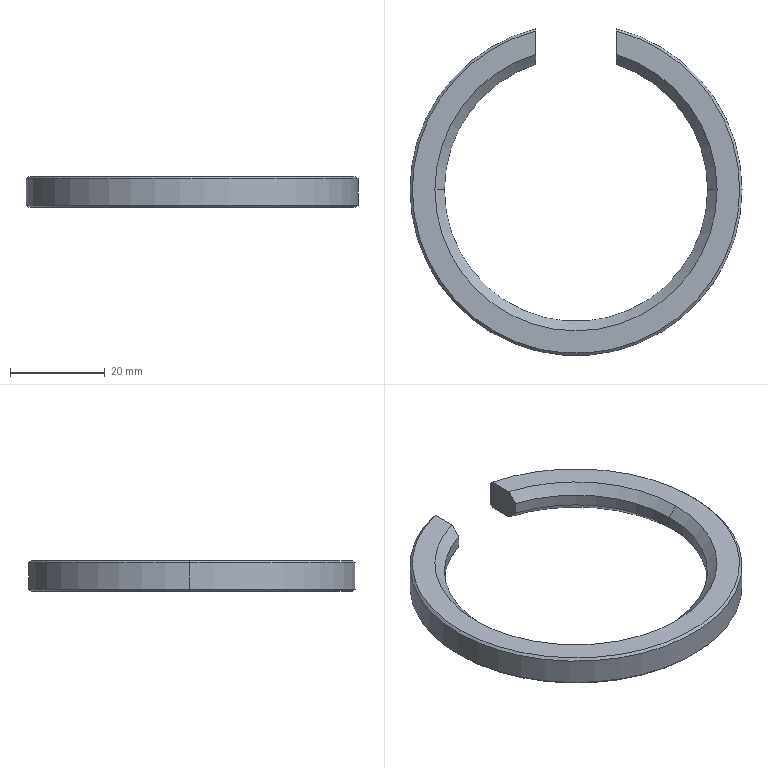Part | SolidWorks | features Chamfer 2, Extrusion 1, ICE 1 | 1 solid | 22 faces | box 70 x 68.952 x 6.5 mm | volume 7783 mm3 | cone 12 | cylinder 6 | plane 4 | commonest cylinder face diameters 55.5 x3 70 x3
STEP:
#1=CARTESIAN_POINT('',(34.5,0.,6.5));
#2=VERTEX_POINT('',#1);
#3=CARTESIAN_POINT('',(8.5,33.437,6.5));
#4=VERTEX_POINT('',#3);
#5=CARTESIAN_POINT('',(0.,0.,6.5));
#6=DIRECTION('',(0.,0.,1.));
#7=DIRECTION('',(1.,0.,0.));
#8=AXIS2_PLACEMENT_3D('',#5,#6,#7);
#9=CIRCLE('',#8,34.5);
#10=EDGE_CURVE('',#2,#4,#9,.T.);
#11=ORIENTED_EDGE('',*,*,#10,.F.);
#12=CARTESIAN_POINT('',(35.,0.,6.));
#13=VERTEX_POINT('',#12);
#14=CARTESIAN_POINT('',(34.5,0.,6.5));
#15=DIRECTION('',(0.7071,0.,-0.7071));
#16=VECTOR('',#15,1000.);
#17=LINE('',#14,#16);
#18=EDGE_CURVE('',#2,#13,#17,.T.);
#19=ORIENTED_EDGE('',*,*,#18,.T.);
#20=CARTESIAN_POINT('',(8.5,33.952,6.));
#21=VERTEX_POINT('',#20);
#22=CARTESIAN_POINT('',(0.,0.,6.));
#23=DIRECTION('',(0.,0.,-1.));
#24=DIRECTION('',(1.,0.,0.));
#25=AXIS2_PLACEMENT_3D('',#22,#23,#24);
#26=CIRCLE('',#25,35.);
#27=EDGE_CURVE('',#21,#13,#26,.T.);
#28=ORIENTED_EDGE('',*,*,#27,.F.);
#29=CARTESIAN_POINT('',(8.5,33.437,6.5));
#30=CARTESIAN_POINT('',(8.5,33.608,6.333));
#31=CARTESIAN_POINT('',(8.5,33.78,6.167));
#32=CARTESIAN_POINT('',(8.5,33.952,6.));
#33=B_SPLINE_CURVE_WITH_KNOTS('',3,(#29,#30,#31,#32),.UNSPECIFIED.,.F.,.F.,(4,4),(0.,0.0007183),.UNSPECIFIED.);
#34=EDGE_CURVE('',#4,#21,#33,.T.);
#35=ORIENTED_EDGE('',*,*,#34,.F.);
#36=EDGE_LOOP('',(#11,#19,#28,#35));
#37=FACE_OUTER_BOUND('',#36,.T.);
#38=CARTESIAN_POINT('',(0.,0.,6.5));
#39=DIRECTION('',(0.,0.,-1.));
#40=DIRECTION('',(-1.,0.,0.));
#41=AXIS2_PLACEMENT_3D('',#38,#39,#40);
#42=CONICAL_SURFACE('',#41,34.5,0.7854);
#43=ADVANCED_FACE('',(#37),#42,.T.);
#44=ORIENTED_EDGE('',*,*,#18,.F.);
#45=CARTESIAN_POINT('',(-34.5,0.,6.5));
#46=VERTEX_POINT('',#45);
#47=CARTESIAN_POINT('',(0.,0.,6.5));
#48=DIRECTION('',(0.,0.,1.));
#49=DIRECTION('',(1.,0.,0.));
#50=AXIS2_PLACEMENT_3D('',#47,#48,#49);
#51=CIRCLE('',#50,34.5);
#52=EDGE_CURVE('',#46,#2,#51,.T.);
#53=ORIENTED_EDGE('',*,*,#52,.F.);
#54=CARTESIAN_POINT('',(-35.,0.,6.));
#55=VERTEX_POINT('',#54);
#56=CARTESIAN_POINT('',(-34.5,0.,6.5));
#57=DIRECTION('',(-0.7071,0.,-0.7071));
#58=VECTOR('',#57,1000.);
#59=LINE('',#56,#58);
#60=EDGE_CURVE('',#46,#55,#59,.T.);
#61=ORIENTED_EDGE('',*,*,#60,.T.);
#62=CARTESIAN_POINT('',(0.,0.,6.));
#63=DIRECTION('',(0.,0.,-1.));
#64=DIRECTION('',(1.,0.,0.));
#65=AXIS2_PLACEMENT_3D('',#62,#63,#64);
#66=CIRCLE('',#65,35.);
#67=EDGE_CURVE('',#13,#55,#66,.T.);
#68=ORIENTED_EDGE('',*,*,#67,.F.);
#69=EDGE_LOOP('',(#44,#53,#61,#68));
#70=FACE_OUTER_BOUND('',#69,.T.);
#71=CARTESIAN_POINT('',(0.,0.,6.5));
#72=DIRECTION('',(0.,0.,-1.));
#73=DIRECTION('',(-1.,0.,0.));
#74=AXIS2_PLACEMENT_3D('',#71,#72,#73);
#75=CONICAL_SURFACE('',#74,34.5,0.7854);
#76=ADVANCED_FACE('',(#70),#75,.T.);
#77=CARTESIAN_POINT('',(-34.5,0.,0.));
#78=VERTEX_POINT('',#77);
#79=CARTESIAN_POINT('',(-8.5,33.437,0.));
#80=VERTEX_POINT('',#79);
#81=CARTESIAN_POINT('',(0.,0.,0.));
#82=DIRECTION('',(0.,0.,-1.));
#83=DIRECTION('',(1.,0.,0.));
#84=AXIS2_PLACEMENT_3D('',#81,#82,#83);
#85=CIRCLE('',#84,34.5);
#86=EDGE_CURVE('',#78,#80,#85,.T.);
#87=ORIENTED_EDGE('',*,*,#86,.F.);
#88=CARTESIAN_POINT('',(-35.,0.,0.5));
#89=VERTEX_POINT('',#88);
#90=CARTESIAN_POINT('',(-35.,0.,0.5));
#91=DIRECTION('',(-0.7071,0.,0.7071));
#92=VECTOR('',#91,1000.);
#93=LINE('',#90,#92);
#94=EDGE_CURVE('',#78,#89,#93,.T.);
#95=ORIENTED_EDGE('',*,*,#94,.T.);
#96=CARTESIAN_POINT('',(-8.5,33.952,0.5));
#97=VERTEX_POINT('',#96);
#98=CARTESIAN_POINT('',(0.,0.,0.5));
#99=DIRECTION('',(0.,0.,1.));
#100=DIRECTION('',(1.,0.,0.));
#101=AXIS2_PLACEMENT_3D('',#98,#99,#100);
#102=CIRCLE('',#101,35.);
#103=EDGE_CURVE('',#97,#89,#102,.T.);
#104=ORIENTED_EDGE('',*,*,#103,.F.);
#105=CARTESIAN_POINT('',(-8.5,33.437,0.));
#106=CARTESIAN_POINT('',(-8.5,33.608,0.1666));
#107=CARTESIAN_POINT('',(-8.5,33.78,0.3333));
#108=CARTESIAN_POINT('',(-8.5,33.952,0.5));
#109=B_SPLINE_CURVE_WITH_KNOTS('',3,(#105,#106,#107,#108),.UNSPECIFIED.,.F.,.F.,(4,4),(0.,0.0007183),.UNSPECIFIED.);
#110=EDGE_CURVE('',#80,#97,#109,.T.);
#111=ORIENTED_EDGE('',*,*,#110,.F.);
#112=EDGE_LOOP('',(#87,#95,#104,#111));
#113=FACE_OUTER_BOUND('',#112,.T.);
#114=CARTESIAN_POINT('',(0.,0.,0.5));
#115=DIRECTION('',(0.,0.,1.));
#116=DIRECTION('',(1.,0.,0.));
#117=AXIS2_PLACEMENT_3D('',#114,#115,#116);
#118=CONICAL_SURFACE('',#117,35.,0.7854);
#119=ADVANCED_FACE('',(#113),#118,.T.);
#120=ORIENTED_EDGE('',*,*,#94,.F.);
#121=CARTESIAN_POINT('',(34.5,0.,0.));
#122=VERTEX_POINT('',#121);
#123=CARTESIAN_POINT('',(0.,0.,0.));
#124=DIRECTION('',(0.,0.,-1.));
#125=DIRECTION('',(1.,0.,0.));
#126=AXIS2_PLACEMENT_3D('',#123,#124,#125);
#127=CIRCLE('',#126,34.5);
#128=EDGE_CURVE('',#122,#78,#127,.T.);
#129=ORIENTED_EDGE('',*,*,#128,.F.);
#130=CARTESIAN_POINT('',(35.,0.,0.5));
#131=VERTEX_POINT('',#130);
#132=CARTESIAN_POINT('',(35.,0.,0.5));
#133=DIRECTION('',(0.7071,0.,0.7071));
#134=VECTOR('',#133,1000.);
#135=LINE('',#132,#134);
#136=EDGE_CURVE('',#122,#131,#135,.T.);
#137=ORIENTED_EDGE('',*,*,#136,.T.);
#138=CARTESIAN_POINT('',(0.,0.,0.5));
#139=DIRECTION('',(0.,0.,1.));
#140=DIRECTION('',(1.,0.,0.));
#141=AXIS2_PLACEMENT_3D('',#138,#139,#140);
#142=CIRCLE('',#141,35.);
#143=EDGE_CURVE('',#89,#131,#142,.T.);
#144=ORIENTED_EDGE('',*,*,#143,.F.);
#145=EDGE_LOOP('',(#120,#129,#137,#144));
#146=FACE_OUTER_BOUND('',#145,.T.);
#147=CARTESIAN_POINT('',(0.,0.,0.5));
#148=DIRECTION('',(0.,0.,1.));
#149=DIRECTION('',(1.,0.,0.));
#150=AXIS2_PLACEMENT_3D('',#147,#148,#149);
#151=CONICAL_SURFACE('',#150,35.,0.7854);
#152=ADVANCED_FACE('',(#146),#151,.T.);
#153=CARTESIAN_POINT('',(-27.75,0.,4.5));
#154=VERTEX_POINT('',#153);
#155=CARTESIAN_POINT('',(27.75,0.,4.5));
#156=VERTEX_POINT('',#155);
#157=CARTESIAN_POINT('',(0.,0.,4.5));
#158=DIRECTION('',(0.,0.,1.));
#159=DIRECTION('',(1.,0.,0.));
#160=AXIS2_PLACEMENT_3D('',#157,#158,#159);
#161=CIRCLE('',#160,27.75);
#162=EDGE_CURVE('',#154,#156,#161,.T.);
#163=ORIENTED_EDGE('',*,*,#162,.F.);
#164=CARTESIAN_POINT('',(-29.75,0.,6.5));
#165=VERTEX_POINT('',#164);
#166=CARTESIAN_POINT('',(-27.75,0.,4.5));
#167=DIRECTION('',(-0.7071,0.,0.7071));
#168=VECTOR('',#167,1000.);
#169=LINE('',#166,#168);
#170=EDGE_CURVE('',#154,#165,#169,.T.);
#171=ORIENTED_EDGE('',*,*,#170,.T.);
#172=CARTESIAN_POINT('',(29.75,0.,6.5));
#173=VERTEX_POINT('',#172);
#174=CARTESIAN_POINT('',(0.,0.,6.5));
#175=DIRECTION('',(0.,0.,-1.));
#176=DIRECTION('',(1.,0.,0.));
#177=AXIS2_PLACEMENT_3D('',#174,#175,#176);
#178=CIRCLE('',#177,29.75);
#179=EDGE_CURVE('',#173,#165,#178,.T.);
#180=ORIENTED_EDGE('',*,*,#179,.F.);
#181=CARTESIAN_POINT('',(27.75,0.,4.5));
#182=DIRECTION('',(0.7071,0.,0.7071));
#183=VECTOR('',#182,1000.);
#184=LINE('',#181,#183);
#185=EDGE_CURVE('',#156,#173,#184,.T.);
#186=ORIENTED_EDGE('',*,*,#185,.F.);
#187=EDGE_LOOP('',(#163,#171,#180,#186));
#188=FACE_OUTER_BOUND('',#187,.T.);
#189=CARTESIAN_POINT('',(0.,0.,4.5));
#190=DIRECTION('',(0.,0.,1.));
#191=DIRECTION('',(1.,0.,0.));
#192=AXIS2_PLACEMENT_3D('',#189,#190,#191);
#193=CONICAL_SURFACE('',#192,27.75,0.7854);
#194=ADVANCED_FACE('',(#188),#193,.F.);
#195=CARTESIAN_POINT('',(8.5,26.416,4.5));
#196=VERTEX_POINT('',#195);
#197=CARTESIAN_POINT('',(0.,0.,4.5));
#198=DIRECTION('',(0.,0.,1.));
#199=DIRECTION('',(1.,0.,0.));
#200=AXIS2_PLACEMENT_3D('',#197,#198,#199);
#201=CIRCLE('',#200,27.75);
#202=EDGE_CURVE('',#156,#196,#201,.T.);
#203=ORIENTED_EDGE('',*,*,#202,.F.);
#204=ORIENTED_EDGE('',*,*,#185,.T.);
#205=CARTESIAN_POINT('',(8.5,28.51,6.5));
#206=VERTEX_POINT('',#205);
#207=CARTESIAN_POINT('',(0.,0.,6.5));
#208=DIRECTION('',(0.,0.,-1.));
#209=DIRECTION('',(1.,0.,0.));
#210=AXIS2_PLACEMENT_3D('',#207,#208,#209);
#211=CIRCLE('',#210,29.75);
#212=EDGE_CURVE('',#206,#173,#211,.T.);
#213=ORIENTED_EDGE('',*,*,#212,.F.);
#214=CARTESIAN_POINT('',(8.5,26.416,4.5));
#215=CARTESIAN_POINT('',(8.5,27.115,5.165));
#216=CARTESIAN_POINT('',(8.5,27.813,5.832));
#217=CARTESIAN_POINT('',(8.5,28.51,6.5));
#218=B_SPLINE_CURVE_WITH_KNOTS('',3,(#214,#215,#216,#217),.UNSPECIFIED.,.F.,.F.,(4,4),(0.,0.002895),.UNSPECIFIED.);
#219=EDGE_CURVE('',#196,#206,#218,.T.);
#220=ORIENTED_EDGE('',*,*,#219,.F.);
#221=EDGE_LOOP('',(#203,#204,#213,#220));
#222=FACE_OUTER_BOUND('',#221,.T.);
#223=CARTESIAN_POINT('',(0.,0.,4.5));
#224=DIRECTION('',(0.,0.,1.));
#225=DIRECTION('',(1.,0.,0.));
#226=AXIS2_PLACEMENT_3D('',#223,#224,#225);
#227=CONICAL_SURFACE('',#226,27.75,0.7854);
#228=ADVANCED_FACE('',(#222),#227,.F.);
#229=CARTESIAN_POINT('',(27.75,0.,2.));
#230=VERTEX_POINT('',#229);
#231=CARTESIAN_POINT('',(-27.75,0.,2.));
#232=VERTEX_POINT('',#231);
#233=CARTESIAN_POINT('',(0.,0.,2.));
#234=DIRECTION('',(0.,0.,-1.));
#235=DIRECTION('',(1.,0.,0.));
#236=AXIS2_PLACEMENT_3D('',#233,#234,#235);
#237=CIRCLE('',#236,27.75);
#238=EDGE_CURVE('',#230,#232,#237,.T.);
#239=ORIENTED_EDGE('',*,*,#238,.F.);
#240=CARTESIAN_POINT('',(29.75,0.,0.));
#241=VERTEX_POINT('',#240);
#242=CARTESIAN_POINT('',(29.75,0.,0.));
#243=DIRECTION('',(0.7071,0.,-0.7071));
#244=VECTOR('',#243,1000.);
#245=LINE('',#242,#244);
#246=EDGE_CURVE('',#230,#241,#245,.T.);
#247=ORIENTED_EDGE('',*,*,#246,.T.);
#248=CARTESIAN_POINT('',(-29.75,0.,0.));
#249=VERTEX_POINT('',#248);
#250=CARTESIAN_POINT('',(0.,0.,0.));
#251=DIRECTION('',(0.,0.,1.));
#252=DIRECTION('',(1.,0.,0.));
#253=AXIS2_PLACEMENT_3D('',#250,#251,#252);
#254=CIRCLE('',#253,29.75);
#255=EDGE_CURVE('',#249,#241,#254,.T.);
#256=ORIENTED_EDGE('',*,*,#255,.F.);
#257=CARTESIAN_POINT('',(-29.75,0.,0.));
#258=DIRECTION('',(-0.7071,0.,-0.7071));
#259=VECTOR('',#258,1000.);
#260=LINE('',#257,#259);
#261=EDGE_CURVE('',#232,#249,#260,.T.);
#262=ORIENTED_EDGE('',*,*,#261,.F.);
#263=EDGE_LOOP('',(#239,#247,#256,#262));
#264=FACE_OUTER_BOUND('',#263,.T.);
#265=CARTESIAN_POINT('',(0.,0.,0.));
#266=DIRECTION('',(0.,0.,-1.));
#267=DIRECTION('',(-1.,0.,0.));
#268=AXIS2_PLACEMENT_3D('',#265,#266,#267);
#269=CONICAL_SURFACE('',#268,29.75,0.7854);
#270=ADVANCED_FACE('',(#264),#269,.F.);
#271=CARTESIAN_POINT('',(-8.5,26.416,2.));
#272=VERTEX_POINT('',#271);
#273=CARTESIAN_POINT('',(0.,0.,2.));
#274=DIRECTION('',(0.,0.,-1.));
#275=DIRECTION('',(1.,0.,0.));
#276=AXIS2_PLACEMENT_3D('',#273,#274,#275);
#277=CIRCLE('',#276,27.75);
#278=EDGE_CURVE('',#232,#272,#277,.T.);
#279=ORIENTED_EDGE('',*,*,#278,.F.);
#280=ORIENTED_EDGE('',*,*,#261,.T.);
#281=CARTESIAN_POINT('',(-8.5,28.51,0.));
#282=VERTEX_POINT('',#281);
#283=CARTESIAN_POINT('',(0.,0.,0.));
#284=DIRECTION('',(0.,0.,1.));
#285=DIRECTION('',(1.,0.,0.));
#286=AXIS2_PLACEMENT_3D('',#283,#284,#285);
#287=CIRCLE('',#286,29.75);
#288=EDGE_CURVE('',#282,#249,#287,.T.);
#289=ORIENTED_EDGE('',*,*,#288,.F.);
#290=CARTESIAN_POINT('',(-8.5,26.416,2.));
#291=CARTESIAN_POINT('',(-8.5,27.115,1.335));
#292=CARTESIAN_POINT('',(-8.5,27.813,0.6678));
#293=CARTESIAN_POINT('',(-8.5,28.51,0.));
#294=B_SPLINE_CURVE_WITH_KNOTS('',3,(#290,#291,#292,#293),.UNSPECIFIED.,.F.,.F.,(4,4),(0.,0.002895),.UNSPECIFIED.);
#295=EDGE_CURVE('',#272,#282,#294,.T.);
#296=ORIENTED_EDGE('',*,*,#295,.F.);
#297=EDGE_LOOP('',(#279,#280,#289,#296));
#298=FACE_OUTER_BOUND('',#297,.T.);
#299=CARTESIAN_POINT('',(0.,0.,0.));
#300=DIRECTION('',(0.,0.,-1.));
#301=DIRECTION('',(-1.,0.,0.));
#302=AXIS2_PLACEMENT_3D('',#299,#300,#301);
#303=CONICAL_SURFACE('',#302,29.75,0.7854);
#304=ADVANCED_FACE('',(#298),#303,.F.);
#305=ORIENTED_EDGE('',*,*,#162,.T.);
#306=CARTESIAN_POINT('',(27.75,0.,6.5));
#307=DIRECTION('',(0.,0.,-1.));
#308=VECTOR('',#307,1000.);
#309=LINE('',#306,#308);
#310=EDGE_CURVE('',#156,#230,#309,.T.);
#311=ORIENTED_EDGE('',*,*,#310,.T.);
#312=ORIENTED_EDGE('',*,*,#238,.T.);
#313=CARTESIAN_POINT('',(-27.75,0.,6.5));
#314=DIRECTION('',(0.,0.,-1.));
#315=VECTOR('',#314,1000.);
#316=LINE('',#313,#315);
#317=EDGE_CURVE('',#154,#232,#316,.T.);
#318=ORIENTED_EDGE('',*,*,#317,.F.);
#319=EDGE_LOOP('',(#305,#311,#312,#318));
#320=FACE_OUTER_BOUND('',#319,.T.);
#321=CARTESIAN_POINT('',(0.,0.,6.5));
#322=DIRECTION('',(0.,0.,-1.));
#323=DIRECTION('',(-1.,0.,0.));
#324=AXIS2_PLACEMENT_3D('',#321,#322,#323);
#325=CYLINDRICAL_SURFACE('',#324,27.75);
#326=ADVANCED_FACE('',(#320),#325,.F.);
#327=CARTESIAN_POINT('',(-8.5,26.416,4.5));
#328=VERTEX_POINT('',#327);
#329=CARTESIAN_POINT('',(0.,0.,4.5));
#330=DIRECTION('',(0.,0.,1.));
#331=DIRECTION('',(1.,0.,0.));
#332=AXIS2_PLACEMENT_3D('',#329,#330,#331);
#333=CIRCLE('',#332,27.75);
#334=EDGE_CURVE('',#328,#154,#333,.T.);
#335=ORIENTED_EDGE('',*,*,#334,.T.);
#336=ORIENTED_EDGE('',*,*,#317,.T.);
#337=ORIENTED_EDGE('',*,*,#278,.T.);
#338=CARTESIAN_POINT('',(-8.5,26.416,6.5));
#339=DIRECTION('',(0.,0.,-1.));
#340=VECTOR('',#339,1000.);
#341=LINE('',#338,#340);
#342=EDGE_CURVE('',#328,#272,#341,.T.);
#343=ORIENTED_EDGE('',*,*,#342,.F.);
#344=EDGE_LOOP('',(#335,#336,#337,#343));
#345=FACE_OUTER_BOUND('',#344,.T.);
#346=CARTESIAN_POINT('',(0.,0.,6.5));
#347=DIRECTION('',(0.,0.,-1.));
#348=DIRECTION('',(-1.,0.,0.));
#349=AXIS2_PLACEMENT_3D('',#346,#347,#348);
#350=CYLINDRICAL_SURFACE('',#349,27.75);
#351=ADVANCED_FACE('',(#345),#350,.F.);
#352=ORIENTED_EDGE('',*,*,#27,.T.);
#353=CARTESIAN_POINT('',(35.,0.,6.5));
#354=DIRECTION('',(0.,0.,-1.));
#355=VECTOR('',#354,1000.);
#356=LINE('',#353,#355);
#357=EDGE_CURVE('',#13,#131,#356,.T.);
#358=ORIENTED_EDGE('',*,*,#357,.T.);
#359=CARTESIAN_POINT('',(8.5,33.952,0.5));
#360=VERTEX_POINT('',#359);
#361=CARTESIAN_POINT('',(0.,0.,0.5));
#362=DIRECTION('',(0.,0.,1.));
#363=DIRECTION('',(1.,0.,0.));
#364=AXIS2_PLACEMENT_3D('',#361,#362,#363);
#365=CIRCLE('',#364,35.);
#366=EDGE_CURVE('',#131,#360,#365,.T.);
#367=ORIENTED_EDGE('',*,*,#366,.T.);
#368=CARTESIAN_POINT('',(8.5,33.952,6.5));
#369=DIRECTION('',(0.,0.,1.));
#370=VECTOR('',#369,1000.);
#371=LINE('',#368,#370);
#372=EDGE_CURVE('',#360,#21,#371,.T.);
#373=ORIENTED_EDGE('',*,*,#372,.T.);
#374=EDGE_LOOP('',(#352,#358,#367,#373));
#375=FACE_OUTER_BOUND('',#374,.T.);
#376=CARTESIAN_POINT('',(0.,0.,6.5));
#377=DIRECTION('',(0.,0.,-1.));
#378=DIRECTION('',(-1.,0.,0.));
#379=AXIS2_PLACEMENT_3D('',#376,#377,#378);
#380=CYLINDRICAL_SURFACE('',#379,35.);
#381=ADVANCED_FACE('',(#375),#380,.T.);
#382=ORIENTED_EDGE('',*,*,#357,.F.);
#383=ORIENTED_EDGE('',*,*,#67,.T.);
#384=CARTESIAN_POINT('',(-35.,0.,6.5));
#385=DIRECTION('',(0.,0.,-1.));
#386=VECTOR('',#385,1000.);
#387=LINE('',#384,#386);
#388=EDGE_CURVE('',#55,#89,#387,.T.);
#389=ORIENTED_EDGE('',*,*,#388,.T.);
#390=ORIENTED_EDGE('',*,*,#143,.T.);
#391=EDGE_LOOP('',(#382,#383,#389,#390));
#392=FACE_OUTER_BOUND('',#391,.T.);
#393=CARTESIAN_POINT('',(0.,0.,6.5));
#394=DIRECTION('',(0.,0.,-1.));
#395=DIRECTION('',(-1.,0.,0.));
#396=AXIS2_PLACEMENT_3D('',#393,#394,#395);
#397=CYLINDRICAL_SURFACE('',#396,35.);
#398=ADVANCED_FACE('',(#392),#397,.T.);
#399=CARTESIAN_POINT('',(-8.5,33.437,6.5));
#400=VERTEX_POINT('',#399);
#401=CARTESIAN_POINT('',(-8.5,28.51,6.5));
#402=VERTEX_POINT('',#401);
#403=CARTESIAN_POINT('',(-8.5,53.905,6.5));
#404=DIRECTION('',(0.,-1.,0.));
#405=VECTOR('',#404,1000.);
#406=LINE('',#403,#405);
#407=EDGE_CURVE('',#400,#402,#406,.T.);
#408=ORIENTED_EDGE('',*,*,#407,.F.);
#409=CARTESIAN_POINT('',(0.,0.,6.5));
#410=DIRECTION('',(0.,0.,1.));
#411=DIRECTION('',(1.,0.,0.));
#412=AXIS2_PLACEMENT_3D('',#409,#410,#411);
#413=CIRCLE('',#412,34.5);
#414=EDGE_CURVE('',#400,#46,#413,.T.);
#415=ORIENTED_EDGE('',*,*,#414,.T.);
#416=ORIENTED_EDGE('',*,*,#52,.T.);
#417=ORIENTED_EDGE('',*,*,#10,.T.);
#418=CARTESIAN_POINT('',(8.5,0.,6.5));
#419=DIRECTION('',(0.,1.,0.));
#420=VECTOR('',#419,1000.);
#421=LINE('',#418,#420);
#422=EDGE_CURVE('',#206,#4,#421,.T.);
#423=ORIENTED_EDGE('',*,*,#422,.F.);
#424=ORIENTED_EDGE('',*,*,#212,.T.);
#425=ORIENTED_EDGE('',*,*,#179,.T.);
#426=CARTESIAN_POINT('',(0.,0.,6.5));
#427=DIRECTION('',(0.,0.,-1.));
#428=DIRECTION('',(1.,0.,0.));
#429=AXIS2_PLACEMENT_3D('',#426,#427,#428);
#430=CIRCLE('',#429,29.75);
#431=EDGE_CURVE('',#165,#402,#430,.T.);
#432=ORIENTED_EDGE('',*,*,#431,.T.);
#433=EDGE_LOOP('',(#408,#415,#416,#417,#423,#424,#425,#432));
#434=FACE_OUTER_BOUND('',#433,.T.);
#435=CARTESIAN_POINT('',(0.,0.,6.5));
#436=DIRECTION('',(0.,0.,1.));
#437=DIRECTION('',(1.,0.,0.));
#438=AXIS2_PLACEMENT_3D('',#435,#436,#437);
#439=PLANE('',#438);
#440=ADVANCED_FACE('',(#434),#439,.T.);
#441=CARTESIAN_POINT('',(8.5,28.51,0.));
#442=VERTEX_POINT('',#441);
#443=CARTESIAN_POINT('',(8.5,33.437,0.));
#444=VERTEX_POINT('',#443);
#445=CARTESIAN_POINT('',(8.5,0.,0.));
#446=DIRECTION('',(0.,1.,0.));
#447=VECTOR('',#446,1000.);
#448=LINE('',#445,#447);
#449=EDGE_CURVE('',#442,#444,#448,.T.);
#450=ORIENTED_EDGE('',*,*,#449,.T.);
#451=CARTESIAN_POINT('',(0.,0.,0.));
#452=DIRECTION('',(0.,0.,-1.));
#453=DIRECTION('',(1.,0.,0.));
#454=AXIS2_PLACEMENT_3D('',#451,#452,#453);
#455=CIRCLE('',#454,34.5);
#456=EDGE_CURVE('',#444,#122,#455,.T.);
#457=ORIENTED_EDGE('',*,*,#456,.T.);
#458=ORIENTED_EDGE('',*,*,#128,.T.);
#459=ORIENTED_EDGE('',*,*,#86,.T.);
#460=CARTESIAN_POINT('',(-8.5,53.905,0.));
#461=DIRECTION('',(0.,-1.,0.));
#462=VECTOR('',#461,1000.);
#463=LINE('',#460,#462);
#464=EDGE_CURVE('',#80,#282,#463,.T.);
#465=ORIENTED_EDGE('',*,*,#464,.T.);
#466=ORIENTED_EDGE('',*,*,#288,.T.);
#467=ORIENTED_EDGE('',*,*,#255,.T.);
#468=CARTESIAN_POINT('',(0.,0.,0.));
#469=DIRECTION('',(0.,0.,1.));
#470=DIRECTION('',(1.,0.,0.));
#471=AXIS2_PLACEMENT_3D('',#468,#469,#470);
#472=CIRCLE('',#471,29.75);
#473=EDGE_CURVE('',#241,#442,#472,.T.);
#474=ORIENTED_EDGE('',*,*,#473,.T.);
#475=EDGE_LOOP('',(#450,#457,#458,#459,#465,#466,#467,#474));
#476=FACE_OUTER_BOUND('',#475,.T.);
#477=CARTESIAN_POINT('',(0.,0.,0.));
#478=DIRECTION('',(0.,0.,1.));
#479=DIRECTION('',(1.,0.,0.));
#480=AXIS2_PLACEMENT_3D('',#477,#478,#479);
#481=PLANE('',#480);
#482=ADVANCED_FACE('',(#476),#481,.F.);
#483=ORIENTED_EDGE('',*,*,#388,.F.);
#484=CARTESIAN_POINT('',(-8.5,33.952,6.));
#485=VERTEX_POINT('',#484);
#486=CARTESIAN_POINT('',(0.,0.,6.));
#487=DIRECTION('',(0.,0.,-1.));
#488=DIRECTION('',(1.,0.,0.));
#489=AXIS2_PLACEMENT_3D('',#486,#487,#488);
#490=CIRCLE('',#489,35.);
#491=EDGE_CURVE('',#55,#485,#490,.T.);
#492=ORIENTED_EDGE('',*,*,#491,.T.);
#493=CARTESIAN_POINT('',(-8.5,33.952,6.5));
#494=DIRECTION('',(0.,0.,-1.));
#495=VECTOR('',#494,1000.);
#496=LINE('',#493,#495);
#497=EDGE_CURVE('',#485,#97,#496,.T.);
#498=ORIENTED_EDGE('',*,*,#497,.T.);
#499=ORIENTED_EDGE('',*,*,#103,.T.);
#500=EDGE_LOOP('',(#483,#492,#498,#499));
#501=FACE_OUTER_BOUND('',#500,.T.);
#502=CARTESIAN_POINT('',(0.,0.,6.5));
#503=DIRECTION('',(0.,0.,-1.));
#504=DIRECTION('',(-1.,0.,0.));
#505=AXIS2_PLACEMENT_3D('',#502,#503,#504);
#506=CYLINDRICAL_SURFACE('',#505,35.);
#507=ADVANCED_FACE('',(#501),#506,.T.);
#508=ORIENTED_EDGE('',*,*,#310,.F.);
#509=ORIENTED_EDGE('',*,*,#202,.T.);
#510=CARTESIAN_POINT('',(8.5,26.416,2.));
#511=VERTEX_POINT('',#510);
#512=CARTESIAN_POINT('',(8.5,26.416,6.5));
#513=DIRECTION('',(0.,0.,1.));
#514=VECTOR('',#513,1000.);
#515=LINE('',#512,#514);
#516=EDGE_CURVE('',#511,#196,#515,.T.);
#517=ORIENTED_EDGE('',*,*,#516,.F.);
#518=CARTESIAN_POINT('',(0.,0.,2.));
#519=DIRECTION('',(0.,0.,-1.));
#520=DIRECTION('',(1.,0.,0.));
#521=AXIS2_PLACEMENT_3D('',#518,#519,#520);
#522=CIRCLE('',#521,27.75);
#523=EDGE_CURVE('',#511,#230,#522,.T.);
#524=ORIENTED_EDGE('',*,*,#523,.T.);
#525=EDGE_LOOP('',(#508,#509,#517,#524));
#526=FACE_OUTER_BOUND('',#525,.T.);
#527=CARTESIAN_POINT('',(0.,0.,6.5));
#528=DIRECTION('',(0.,0.,-1.));
#529=DIRECTION('',(-1.,0.,0.));
#530=AXIS2_PLACEMENT_3D('',#527,#528,#529);
#531=CYLINDRICAL_SURFACE('',#530,27.75);
#532=ADVANCED_FACE('',(#526),#531,.F.);
#533=ORIENTED_EDGE('',*,*,#372,.F.);
#534=CARTESIAN_POINT('',(8.5,33.952,0.5));
#535=CARTESIAN_POINT('',(8.5,33.78,0.3333));
#536=CARTESIAN_POINT('',(8.5,33.608,0.1666));
#537=CARTESIAN_POINT('',(8.5,33.437,0.));
#538=B_SPLINE_CURVE_WITH_KNOTS('',3,(#534,#535,#536,#537),.UNSPECIFIED.,.F.,.F.,(4,4),(0.,0.0007183),.UNSPECIFIED.);
#539=EDGE_CURVE('',#360,#444,#538,.T.);
#540=ORIENTED_EDGE('',*,*,#539,.T.);
#541=ORIENTED_EDGE('',*,*,#449,.F.);
#542=CARTESIAN_POINT('',(8.5,28.51,0.));
#543=CARTESIAN_POINT('',(8.5,27.813,0.6678));
#544=CARTESIAN_POINT('',(8.5,27.115,1.335));
#545=CARTESIAN_POINT('',(8.5,26.416,2.));
#546=B_SPLINE_CURVE_WITH_KNOTS('',3,(#542,#543,#544,#545),.UNSPECIFIED.,.F.,.F.,(4,4),(0.,0.002895),.UNSPECIFIED.);
#547=EDGE_CURVE('',#442,#511,#546,.T.);
#548=ORIENTED_EDGE('',*,*,#547,.T.);
#549=ORIENTED_EDGE('',*,*,#516,.T.);
#550=ORIENTED_EDGE('',*,*,#219,.T.);
#551=ORIENTED_EDGE('',*,*,#422,.T.);
#552=ORIENTED_EDGE('',*,*,#34,.T.);
#553=EDGE_LOOP('',(#533,#540,#541,#548,#549,#550,#551,#552));
#554=FACE_OUTER_BOUND('',#553,.T.);
#555=CARTESIAN_POINT('',(8.5,0.,0.));
#556=DIRECTION('',(1.,0.,0.));
#557=DIRECTION('',(0.,0.,-1.));
#558=AXIS2_PLACEMENT_3D('',#555,#556,#557);
#559=PLANE('',#558);
#560=ADVANCED_FACE('',(#554),#559,.F.);
#561=ORIENTED_EDGE('',*,*,#464,.F.);
#562=ORIENTED_EDGE('',*,*,#110,.T.);
#563=ORIENTED_EDGE('',*,*,#497,.F.);
#564=CARTESIAN_POINT('',(-8.5,33.952,6.));
#565=CARTESIAN_POINT('',(-8.5,33.78,6.167));
#566=CARTESIAN_POINT('',(-8.5,33.608,6.333));
#567=CARTESIAN_POINT('',(-8.5,33.437,6.5));
#568=B_SPLINE_CURVE_WITH_KNOTS('',3,(#564,#565,#566,#567),.UNSPECIFIED.,.F.,.F.,(4,4),(0.,0.0007183),.UNSPECIFIED.);
#569=EDGE_CURVE('',#485,#400,#568,.T.);
#570=ORIENTED_EDGE('',*,*,#569,.T.);
#571=ORIENTED_EDGE('',*,*,#407,.T.);
#572=CARTESIAN_POINT('',(-8.5,28.51,6.5));
#573=CARTESIAN_POINT('',(-8.5,27.813,5.832));
#574=CARTESIAN_POINT('',(-8.5,27.115,5.165));
#575=CARTESIAN_POINT('',(-8.5,26.416,4.5));
#576=B_SPLINE_CURVE_WITH_KNOTS('',3,(#572,#573,#574,#575),.UNSPECIFIED.,.F.,.F.,(4,4),(0.,0.002895),.UNSPECIFIED.);
#577=EDGE_CURVE('',#402,#328,#576,.T.);
#578=ORIENTED_EDGE('',*,*,#577,.T.);
#579=ORIENTED_EDGE('',*,*,#342,.T.);
#580=ORIENTED_EDGE('',*,*,#295,.T.);
#581=EDGE_LOOP('',(#561,#562,#563,#570,#571,#578,#579,#580));
#582=FACE_OUTER_BOUND('',#581,.T.);
#583=CARTESIAN_POINT('',(-8.5,53.905,0.));
#584=DIRECTION('',(-1.,0.,0.));
#585=DIRECTION('',(0.,-1.,0.));
#586=AXIS2_PLACEMENT_3D('',#583,#584,#585);
#587=PLANE('',#586);
#588=ADVANCED_FACE('',(#582),#587,.F.);
#589=ORIENTED_EDGE('',*,*,#246,.F.);
#590=ORIENTED_EDGE('',*,*,#523,.F.);
#591=ORIENTED_EDGE('',*,*,#547,.F.);
#592=ORIENTED_EDGE('',*,*,#473,.F.);
#593=EDGE_LOOP('',(#589,#590,#591,#592));
#594=FACE_OUTER_BOUND('',#593,.T.);
#595=CARTESIAN_POINT('',(0.,0.,0.));
#596=DIRECTION('',(0.,0.,-1.));
#597=DIRECTION('',(-1.,0.,0.));
#598=AXIS2_PLACEMENT_3D('',#595,#596,#597);
#599=CONICAL_SURFACE('',#598,29.75,0.7854);
#600=ADVANCED_FACE('',(#594),#599,.F.);
#601=ORIENTED_EDGE('',*,*,#170,.F.);
#602=ORIENTED_EDGE('',*,*,#334,.F.);
#603=ORIENTED_EDGE('',*,*,#577,.F.);
#604=ORIENTED_EDGE('',*,*,#431,.F.);
#605=EDGE_LOOP('',(#601,#602,#603,#604));
#606=FACE_OUTER_BOUND('',#605,.T.);
#607=CARTESIAN_POINT('',(0.,0.,4.5));
#608=DIRECTION('',(0.,0.,1.));
#609=DIRECTION('',(1.,0.,0.));
#610=AXIS2_PLACEMENT_3D('',#607,#608,#609);
#611=CONICAL_SURFACE('',#610,27.75,0.7854);
#612=ADVANCED_FACE('',(#606),#611,.F.);
#613=ORIENTED_EDGE('',*,*,#136,.F.);
#614=ORIENTED_EDGE('',*,*,#456,.F.);
#615=ORIENTED_EDGE('',*,*,#539,.F.);
#616=ORIENTED_EDGE('',*,*,#366,.F.);
#617=EDGE_LOOP('',(#613,#614,#615,#616));
#618=FACE_OUTER_BOUND('',#617,.T.);
#619=CARTESIAN_POINT('',(0.,0.,0.5));
#620=DIRECTION('',(0.,0.,1.));
#621=DIRECTION('',(1.,0.,0.));
#622=AXIS2_PLACEMENT_3D('',#619,#620,#621);
#623=CONICAL_SURFACE('',#622,35.,0.7854);
#624=ADVANCED_FACE('',(#618),#623,.T.);
#625=ORIENTED_EDGE('',*,*,#60,.F.);
#626=ORIENTED_EDGE('',*,*,#414,.F.);
#627=ORIENTED_EDGE('',*,*,#569,.F.);
#628=ORIENTED_EDGE('',*,*,#491,.F.);
#629=EDGE_LOOP('',(#625,#626,#627,#628));
#630=FACE_OUTER_BOUND('',#629,.T.);
#631=CARTESIAN_POINT('',(0.,0.,6.5));
#632=DIRECTION('',(0.,0.,-1.));
#633=DIRECTION('',(-1.,0.,0.));
#634=AXIS2_PLACEMENT_3D('',#631,#632,#633);
#635=CONICAL_SURFACE('',#634,34.5,0.7854);
#636=ADVANCED_FACE('',(#630),#635,.T.);
#637=CLOSED_SHELL('',(#43,#76,#119,#152,#194,#228,#270,#304,#326,#351,#381,#398,#440,#482,#507,#532,#560,#588,#600,#612,#624,#636));
#638=MANIFOLD_SOLID_BREP('',#637);
#639=CARTESIAN_POINT('',(0.,0.,0.));
#640=DIRECTION('',(0.,0.,1.));
#641=DIRECTION('',(1.,0.,0.));
#642=AXIS2_PLACEMENT_3D('',#639,#640,#641);
#643=(LENGTH_UNIT()NAMED_UNIT(*)SI_UNIT(.MILLI.,.METRE.));
#644=UNCERTAINTY_MEASURE_WITH_UNIT(LENGTH_MEASURE(0.00001),#643,'','');
#645=(NAMED_UNIT(*)PLANE_ANGLE_UNIT()SI_UNIT($,.RADIAN.));
#646=(NAMED_UNIT(*)SI_UNIT($,.STERADIAN.)SOLID_ANGLE_UNIT());
#647=(GEOMETRIC_REPRESENTATION_CONTEXT(3)GLOBAL_UNCERTAINTY_ASSIGNED_CONTEXT((#644))GLOBAL_UNIT_ASSIGNED_CONTEXT((#643,#645,#646))REPRESENTATION_CONTEXT('',''));
#648=ADVANCED_BREP_SHAPE_REPRESENTATION('',(#638,#642),#647);